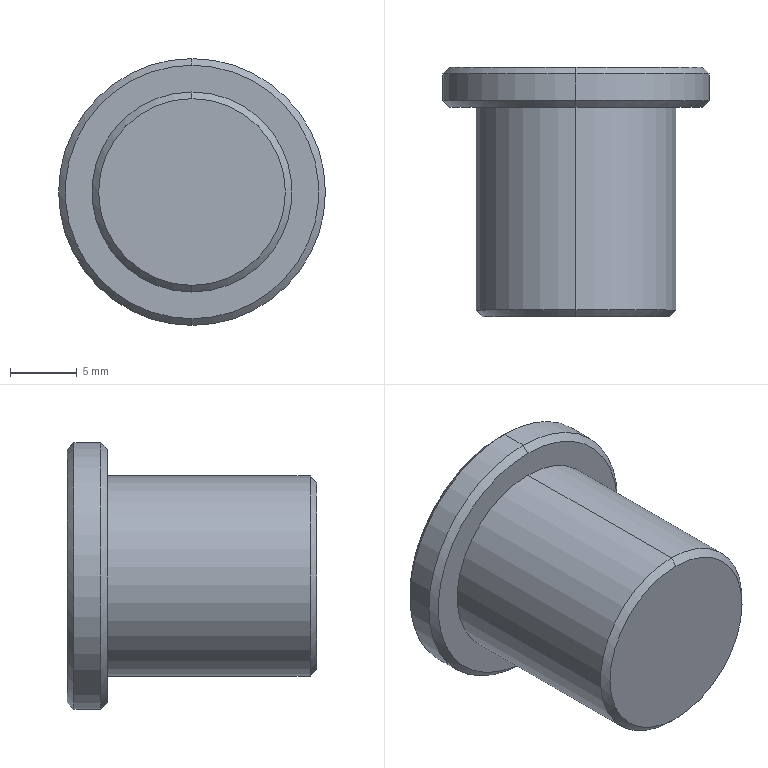Part | SolidWorks | features Chamfer 1, Revolution 1 | 1 solid | 13 faces | box 20 x 18.7 x 20 mm | volume 3696 mm3 | cone 6 | cylinder 4 | plane 3 | commonest cylinder face diameters 15 x2 20 x2
STEP:
#1=CARTESIAN_POINT('',(1016.5,204.199,-7.));
#2=VERTEX_POINT('',#1);
#3=CARTESIAN_POINT('',(1016.5,204.199,7.));
#4=VERTEX_POINT('',#3);
#5=CARTESIAN_POINT('',(1016.5,204.199,0.));
#6=DIRECTION('',(0.,-1.,0.));
#7=DIRECTION('',(0.,0.,-1.));
#8=AXIS2_PLACEMENT_3D('',#5,#6,#7);
#9=CIRCLE('',#8,7.);
#10=EDGE_CURVE('',#2,#4,#9,.T.);
#11=ORIENTED_EDGE('',*,*,#10,.F.);
#12=CARTESIAN_POINT('',(1016.5,204.699,-7.5));
#13=VERTEX_POINT('',#12);
#14=CARTESIAN_POINT('',(1016.5,204.699,-7.5));
#15=DIRECTION('',(0.,0.7071,-0.7071));
#16=VECTOR('',#15,1000.);
#17=LINE('',#14,#16);
#18=EDGE_CURVE('',#2,#13,#17,.T.);
#19=ORIENTED_EDGE('',*,*,#18,.T.);
#20=CARTESIAN_POINT('',(1016.5,204.699,7.5));
#21=VERTEX_POINT('',#20);
#22=CARTESIAN_POINT('',(1016.5,204.699,0.));
#23=DIRECTION('',(0.,1.,0.));
#24=DIRECTION('',(0.,0.,-1.));
#25=AXIS2_PLACEMENT_3D('',#22,#23,#24);
#26=CIRCLE('',#25,7.5);
#27=EDGE_CURVE('',#21,#13,#26,.T.);
#28=ORIENTED_EDGE('',*,*,#27,.F.);
#29=CARTESIAN_POINT('',(1016.5,204.699,7.5));
#30=DIRECTION('',(0.,0.7071,0.7071));
#31=VECTOR('',#30,1000.);
#32=LINE('',#29,#31);
#33=EDGE_CURVE('',#4,#21,#32,.T.);
#34=ORIENTED_EDGE('',*,*,#33,.F.);
#35=EDGE_LOOP('',(#11,#19,#28,#34));
#36=FACE_OUTER_BOUND('',#35,.T.);
#37=CARTESIAN_POINT('',(1016.5,204.699,0.));
#38=DIRECTION('',(0.,1.,0.));
#39=DIRECTION('',(0.,0.,1.));
#40=AXIS2_PLACEMENT_3D('',#37,#38,#39);
#41=CONICAL_SURFACE('',#40,7.5,0.7854);
#42=ADVANCED_FACE('',(#36),#41,.T.);
#43=CARTESIAN_POINT('',(1016.5,219.899,-9.5));
#44=VERTEX_POINT('',#43);
#45=CARTESIAN_POINT('',(1016.5,219.899,9.5));
#46=VERTEX_POINT('',#45);
#47=CARTESIAN_POINT('',(1016.5,219.899,0.));
#48=DIRECTION('',(0.,-1.,0.));
#49=DIRECTION('',(0.,0.,-1.));
#50=AXIS2_PLACEMENT_3D('',#47,#48,#49);
#51=CIRCLE('',#50,9.5);
#52=EDGE_CURVE('',#44,#46,#51,.T.);
#53=ORIENTED_EDGE('',*,*,#52,.F.);
#54=CARTESIAN_POINT('',(1016.5,220.399,-10.));
#55=VERTEX_POINT('',#54);
#56=CARTESIAN_POINT('',(1016.5,220.399,-10.));
#57=DIRECTION('',(0.,0.7071,-0.7071));
#58=VECTOR('',#57,1000.);
#59=LINE('',#56,#58);
#60=EDGE_CURVE('',#44,#55,#59,.T.);
#61=ORIENTED_EDGE('',*,*,#60,.T.);
#62=CARTESIAN_POINT('',(1016.5,220.399,10.));
#63=VERTEX_POINT('',#62);
#64=CARTESIAN_POINT('',(1016.5,220.399,0.));
#65=DIRECTION('',(0.,1.,0.));
#66=DIRECTION('',(0.,0.,-1.));
#67=AXIS2_PLACEMENT_3D('',#64,#65,#66);
#68=CIRCLE('',#67,10.);
#69=EDGE_CURVE('',#63,#55,#68,.T.);
#70=ORIENTED_EDGE('',*,*,#69,.F.);
#71=CARTESIAN_POINT('',(1016.5,220.399,10.));
#72=DIRECTION('',(0.,0.7071,0.7071));
#73=VECTOR('',#72,1000.);
#74=LINE('',#71,#73);
#75=EDGE_CURVE('',#46,#63,#74,.T.);
#76=ORIENTED_EDGE('',*,*,#75,.F.);
#77=EDGE_LOOP('',(#53,#61,#70,#76));
#78=FACE_OUTER_BOUND('',#77,.T.);
#79=CARTESIAN_POINT('',(1016.5,220.399,0.));
#80=DIRECTION('',(0.,1.,0.));
#81=DIRECTION('',(0.,0.,1.));
#82=AXIS2_PLACEMENT_3D('',#79,#80,#81);
#83=CONICAL_SURFACE('',#82,10.,0.7854);
#84=ADVANCED_FACE('',(#78),#83,.T.);
#85=CARTESIAN_POINT('',(1016.5,222.899,9.5));
#86=VERTEX_POINT('',#85);
#87=CARTESIAN_POINT('',(1016.5,222.899,-9.5));
#88=VERTEX_POINT('',#87);
#89=CARTESIAN_POINT('',(1016.5,222.899,0.));
#90=DIRECTION('',(0.,1.,0.));
#91=DIRECTION('',(0.,0.,1.));
#92=AXIS2_PLACEMENT_3D('',#89,#90,#91);
#93=CIRCLE('',#92,9.5);
#94=EDGE_CURVE('',#86,#88,#93,.T.);
#95=ORIENTED_EDGE('',*,*,#94,.F.);
#96=CARTESIAN_POINT('',(1016.5,222.399,10.));
#97=VERTEX_POINT('',#96);
#98=CARTESIAN_POINT('',(1016.5,222.899,9.5));
#99=DIRECTION('',(0.,-0.7071,0.7071));
#100=VECTOR('',#99,1000.);
#101=LINE('',#98,#100);
#102=EDGE_CURVE('',#86,#97,#101,.T.);
#103=ORIENTED_EDGE('',*,*,#102,.T.);
#104=CARTESIAN_POINT('',(1016.5,222.399,-10.));
#105=VERTEX_POINT('',#104);
#106=CARTESIAN_POINT('',(1016.5,222.399,0.));
#107=DIRECTION('',(0.,-1.,0.));
#108=DIRECTION('',(0.,0.,1.));
#109=AXIS2_PLACEMENT_3D('',#106,#107,#108);
#110=CIRCLE('',#109,10.);
#111=EDGE_CURVE('',#105,#97,#110,.T.);
#112=ORIENTED_EDGE('',*,*,#111,.F.);
#113=CARTESIAN_POINT('',(1016.5,222.899,-9.5));
#114=DIRECTION('',(0.,-0.7071,-0.7071));
#115=VECTOR('',#114,1000.);
#116=LINE('',#113,#115);
#117=EDGE_CURVE('',#88,#105,#116,.T.);
#118=ORIENTED_EDGE('',*,*,#117,.F.);
#119=EDGE_LOOP('',(#95,#103,#112,#118));
#120=FACE_OUTER_BOUND('',#119,.T.);
#121=CARTESIAN_POINT('',(1016.5,222.899,0.));
#122=DIRECTION('',(0.,-1.,0.));
#123=DIRECTION('',(0.,0.,-1.));
#124=AXIS2_PLACEMENT_3D('',#121,#122,#123);
#125=CONICAL_SURFACE('',#124,9.5,0.7854);
#126=ADVANCED_FACE('',(#120),#125,.T.);
#127=ORIENTED_EDGE('',*,*,#69,.T.);
#128=CARTESIAN_POINT('',(1016.5,222.899,-10.));
#129=DIRECTION('',(0.,1.,0.));
#130=VECTOR('',#129,1000.);
#131=LINE('',#128,#130);
#132=EDGE_CURVE('',#55,#105,#131,.T.);
#133=ORIENTED_EDGE('',*,*,#132,.T.);
#134=ORIENTED_EDGE('',*,*,#111,.T.);
#135=CARTESIAN_POINT('',(1016.5,222.899,10.));
#136=DIRECTION('',(0.,1.,0.));
#137=VECTOR('',#136,1000.);
#138=LINE('',#135,#137);
#139=EDGE_CURVE('',#63,#97,#138,.T.);
#140=ORIENTED_EDGE('',*,*,#139,.F.);
#141=EDGE_LOOP('',(#127,#133,#134,#140));
#142=FACE_OUTER_BOUND('',#141,.T.);
#143=CARTESIAN_POINT('',(1016.5,222.899,0.));
#144=DIRECTION('',(0.,1.,0.));
#145=DIRECTION('',(0.,0.,1.));
#146=AXIS2_PLACEMENT_3D('',#143,#144,#145);
#147=CYLINDRICAL_SURFACE('',#146,10.);
#148=ADVANCED_FACE('',(#142),#147,.T.);
#149=ORIENTED_EDGE('',*,*,#27,.T.);
#150=CARTESIAN_POINT('',(1016.5,219.899,-7.5));
#151=VERTEX_POINT('',#150);
#152=CARTESIAN_POINT('',(1016.5,222.899,-7.5));
#153=DIRECTION('',(0.,1.,0.));
#154=VECTOR('',#153,1000.);
#155=LINE('',#152,#154);
#156=EDGE_CURVE('',#13,#151,#155,.T.);
#157=ORIENTED_EDGE('',*,*,#156,.T.);
#158=CARTESIAN_POINT('',(1016.5,219.899,7.5));
#159=VERTEX_POINT('',#158);
#160=CARTESIAN_POINT('',(1016.5,219.899,0.));
#161=DIRECTION('',(0.,1.,0.));
#162=DIRECTION('',(0.,0.,1.));
#163=AXIS2_PLACEMENT_3D('',#160,#161,#162);
#164=CIRCLE('',#163,7.5);
#165=EDGE_CURVE('',#159,#151,#164,.T.);
#166=ORIENTED_EDGE('',*,*,#165,.F.);
#167=CARTESIAN_POINT('',(1016.5,222.899,7.5));
#168=DIRECTION('',(0.,1.,0.));
#169=VECTOR('',#168,1000.);
#170=LINE('',#167,#169);
#171=EDGE_CURVE('',#21,#159,#170,.T.);
#172=ORIENTED_EDGE('',*,*,#171,.F.);
#173=EDGE_LOOP('',(#149,#157,#166,#172));
#174=FACE_OUTER_BOUND('',#173,.T.);
#175=CARTESIAN_POINT('',(1016.5,222.899,0.));
#176=DIRECTION('',(0.,1.,0.));
#177=DIRECTION('',(0.,0.,1.));
#178=AXIS2_PLACEMENT_3D('',#175,#176,#177);
#179=CYLINDRICAL_SURFACE('',#178,7.5);
#180=ADVANCED_FACE('',(#174),#179,.T.);
#181=CARTESIAN_POINT('',(1016.5,204.199,0.));
#182=DIRECTION('',(0.,-1.,0.));
#183=DIRECTION('',(0.,0.,-1.));
#184=AXIS2_PLACEMENT_3D('',#181,#182,#183);
#185=CIRCLE('',#184,7.);
#186=EDGE_CURVE('',#4,#2,#185,.T.);
#187=ORIENTED_EDGE('',*,*,#186,.T.);
#188=ORIENTED_EDGE('',*,*,#10,.T.);
#189=EDGE_LOOP('',(#187,#188));
#190=FACE_OUTER_BOUND('',#189,.T.);
#191=CARTESIAN_POINT('',(1009.,204.199,0.));
#192=DIRECTION('',(0.,-1.,0.));
#193=DIRECTION('',(0.,0.,-1.));
#194=AXIS2_PLACEMENT_3D('',#191,#192,#193);
#195=PLANE('',#194);
#196=ADVANCED_FACE('',(#190),#195,.T.);
#197=ORIENTED_EDGE('',*,*,#156,.F.);
#198=CARTESIAN_POINT('',(1016.5,204.699,0.));
#199=DIRECTION('',(0.,1.,0.));
#200=DIRECTION('',(0.,0.,-1.));
#201=AXIS2_PLACEMENT_3D('',#198,#199,#200);
#202=CIRCLE('',#201,7.5);
#203=EDGE_CURVE('',#13,#21,#202,.T.);
#204=ORIENTED_EDGE('',*,*,#203,.T.);
#205=ORIENTED_EDGE('',*,*,#171,.T.);
#206=CARTESIAN_POINT('',(1016.5,219.899,0.));
#207=DIRECTION('',(0.,1.,0.));
#208=DIRECTION('',(0.,0.,1.));
#209=AXIS2_PLACEMENT_3D('',#206,#207,#208);
#210=CIRCLE('',#209,7.5);
#211=EDGE_CURVE('',#151,#159,#210,.T.);
#212=ORIENTED_EDGE('',*,*,#211,.F.);
#213=EDGE_LOOP('',(#197,#204,#205,#212));
#214=FACE_OUTER_BOUND('',#213,.T.);
#215=CARTESIAN_POINT('',(1016.5,222.899,0.));
#216=DIRECTION('',(0.,1.,0.));
#217=DIRECTION('',(0.,0.,1.));
#218=AXIS2_PLACEMENT_3D('',#215,#216,#217);
#219=CYLINDRICAL_SURFACE('',#218,7.5);
#220=ADVANCED_FACE('',(#214),#219,.T.);
#221=CARTESIAN_POINT('',(1016.5,219.899,0.));
#222=DIRECTION('',(0.,-1.,0.));
#223=DIRECTION('',(0.,0.,-1.));
#224=AXIS2_PLACEMENT_3D('',#221,#222,#223);
#225=CIRCLE('',#224,9.5);
#226=EDGE_CURVE('',#46,#44,#225,.T.);
#227=ORIENTED_EDGE('',*,*,#226,.T.);
#228=ORIENTED_EDGE('',*,*,#52,.T.);
#229=EDGE_LOOP('',(#227,#228));
#230=FACE_OUTER_BOUND('',#229,.T.);
#231=ORIENTED_EDGE('',*,*,#165,.T.);
#232=ORIENTED_EDGE('',*,*,#211,.T.);
#233=EDGE_LOOP('',(#231,#232));
#234=FACE_BOUND('',#233,.T.);
#235=CARTESIAN_POINT('',(1009.,219.899,0.));
#236=DIRECTION('',(0.,-1.,0.));
#237=DIRECTION('',(0.,0.,-1.));
#238=AXIS2_PLACEMENT_3D('',#235,#236,#237);
#239=PLANE('',#238);
#240=ADVANCED_FACE('',(#230,#234),#239,.T.);
#241=ORIENTED_EDGE('',*,*,#132,.F.);
#242=CARTESIAN_POINT('',(1016.5,220.399,0.));
#243=DIRECTION('',(0.,1.,0.));
#244=DIRECTION('',(0.,0.,-1.));
#245=AXIS2_PLACEMENT_3D('',#242,#243,#244);
#246=CIRCLE('',#245,10.);
#247=EDGE_CURVE('',#55,#63,#246,.T.);
#248=ORIENTED_EDGE('',*,*,#247,.T.);
#249=ORIENTED_EDGE('',*,*,#139,.T.);
#250=CARTESIAN_POINT('',(1016.5,222.399,0.));
#251=DIRECTION('',(0.,-1.,0.));
#252=DIRECTION('',(0.,0.,1.));
#253=AXIS2_PLACEMENT_3D('',#250,#251,#252);
#254=CIRCLE('',#253,10.);
#255=EDGE_CURVE('',#97,#105,#254,.T.);
#256=ORIENTED_EDGE('',*,*,#255,.T.);
#257=EDGE_LOOP('',(#241,#248,#249,#256));
#258=FACE_OUTER_BOUND('',#257,.T.);
#259=CARTESIAN_POINT('',(1016.5,222.899,0.));
#260=DIRECTION('',(0.,1.,0.));
#261=DIRECTION('',(0.,0.,1.));
#262=AXIS2_PLACEMENT_3D('',#259,#260,#261);
#263=CYLINDRICAL_SURFACE('',#262,10.);
#264=ADVANCED_FACE('',(#258),#263,.T.);
#265=CARTESIAN_POINT('',(1016.5,222.899,0.));
#266=DIRECTION('',(0.,1.,0.));
#267=DIRECTION('',(0.,0.,1.));
#268=AXIS2_PLACEMENT_3D('',#265,#266,#267);
#269=CIRCLE('',#268,9.5);
#270=EDGE_CURVE('',#88,#86,#269,.T.);
#271=ORIENTED_EDGE('',*,*,#270,.T.);
#272=ORIENTED_EDGE('',*,*,#94,.T.);
#273=EDGE_LOOP('',(#271,#272));
#274=FACE_OUTER_BOUND('',#273,.T.);
#275=CARTESIAN_POINT('',(1006.5,222.899,0.));
#276=DIRECTION('',(0.,1.,0.));
#277=DIRECTION('',(0.,0.,1.));
#278=AXIS2_PLACEMENT_3D('',#275,#276,#277);
#279=PLANE('',#278);
#280=ADVANCED_FACE('',(#274),#279,.T.);
#281=ORIENTED_EDGE('',*,*,#102,.F.);
#282=ORIENTED_EDGE('',*,*,#270,.F.);
#283=ORIENTED_EDGE('',*,*,#117,.T.);
#284=ORIENTED_EDGE('',*,*,#255,.F.);
#285=EDGE_LOOP('',(#281,#282,#283,#284));
#286=FACE_OUTER_BOUND('',#285,.T.);
#287=CARTESIAN_POINT('',(1016.5,222.899,0.));
#288=DIRECTION('',(0.,-1.,0.));
#289=DIRECTION('',(0.,0.,-1.));
#290=AXIS2_PLACEMENT_3D('',#287,#288,#289);
#291=CONICAL_SURFACE('',#290,9.5,0.7854);
#292=ADVANCED_FACE('',(#286),#291,.T.);
#293=ORIENTED_EDGE('',*,*,#60,.F.);
#294=ORIENTED_EDGE('',*,*,#226,.F.);
#295=ORIENTED_EDGE('',*,*,#75,.T.);
#296=ORIENTED_EDGE('',*,*,#247,.F.);
#297=EDGE_LOOP('',(#293,#294,#295,#296));
#298=FACE_OUTER_BOUND('',#297,.T.);
#299=CARTESIAN_POINT('',(1016.5,220.399,0.));
#300=DIRECTION('',(0.,1.,0.));
#301=DIRECTION('',(0.,0.,1.));
#302=AXIS2_PLACEMENT_3D('',#299,#300,#301);
#303=CONICAL_SURFACE('',#302,10.,0.7854);
#304=ADVANCED_FACE('',(#298),#303,.T.);
#305=ORIENTED_EDGE('',*,*,#18,.F.);
#306=ORIENTED_EDGE('',*,*,#186,.F.);
#307=ORIENTED_EDGE('',*,*,#33,.T.);
#308=ORIENTED_EDGE('',*,*,#203,.F.);
#309=EDGE_LOOP('',(#305,#306,#307,#308));
#310=FACE_OUTER_BOUND('',#309,.T.);
#311=CARTESIAN_POINT('',(1016.5,204.699,0.));
#312=DIRECTION('',(0.,1.,0.));
#313=DIRECTION('',(0.,0.,1.));
#314=AXIS2_PLACEMENT_3D('',#311,#312,#313);
#315=CONICAL_SURFACE('',#314,7.5,0.7854);
#316=ADVANCED_FACE('',(#310),#315,.T.);
#317=CLOSED_SHELL('',(#42,#84,#126,#148,#180,#196,#220,#240,#264,#280,#292,#304,#316));
#318=MANIFOLD_SOLID_BREP('',#317);
#319=CARTESIAN_POINT('',(0.,0.,0.));
#320=DIRECTION('',(0.,0.,1.));
#321=DIRECTION('',(1.,0.,0.));
#322=AXIS2_PLACEMENT_3D('',#319,#320,#321);
#323=(LENGTH_UNIT()NAMED_UNIT(*)SI_UNIT(.MILLI.,.METRE.));
#324=UNCERTAINTY_MEASURE_WITH_UNIT(LENGTH_MEASURE(0.00001),#323,'','');
#325=(NAMED_UNIT(*)PLANE_ANGLE_UNIT()SI_UNIT($,.RADIAN.));
#326=(NAMED_UNIT(*)SI_UNIT($,.STERADIAN.)SOLID_ANGLE_UNIT());
#327=(GEOMETRIC_REPRESENTATION_CONTEXT(3)GLOBAL_UNCERTAINTY_ASSIGNED_CONTEXT((#324))GLOBAL_UNIT_ASSIGNED_CONTEXT((#323,#325,#326))REPRESENTATION_CONTEXT('',''));
#328=ADVANCED_BREP_SHAPE_REPRESENTATION('',(#318,#322),#327);